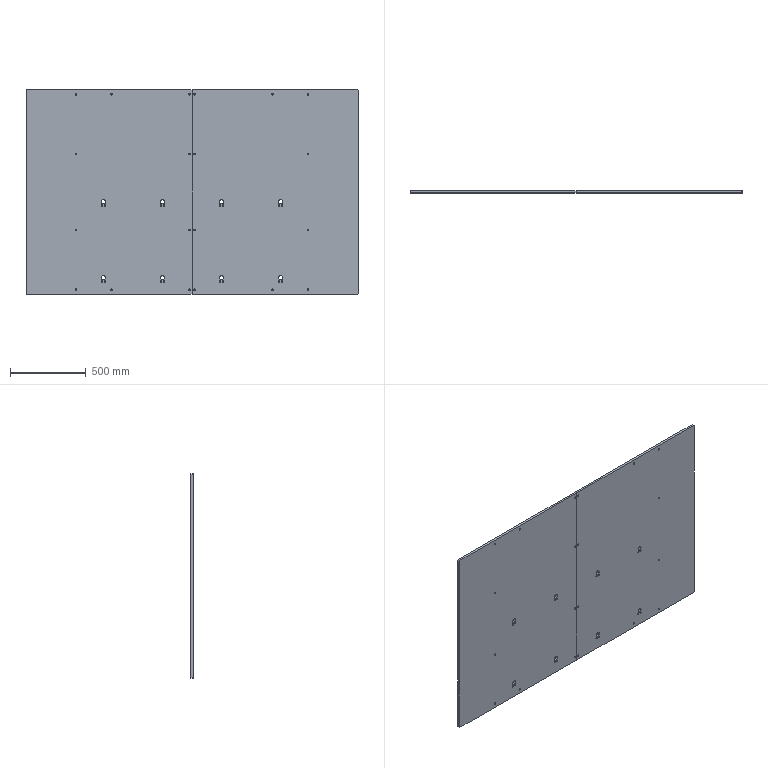Part | SolidWorks | features HoleWzd 3, Chamfer 1, Extrusion 1, PLine 1 | 1 solid | 210 faces | box 2190 x 15 x 1350 mm | volume 44243626 mm3 | cylinder 160 | plane 50 | commonest cylinder face diameters 6.6 x40 11 x40 5.5 x32 10 x32 28 x16